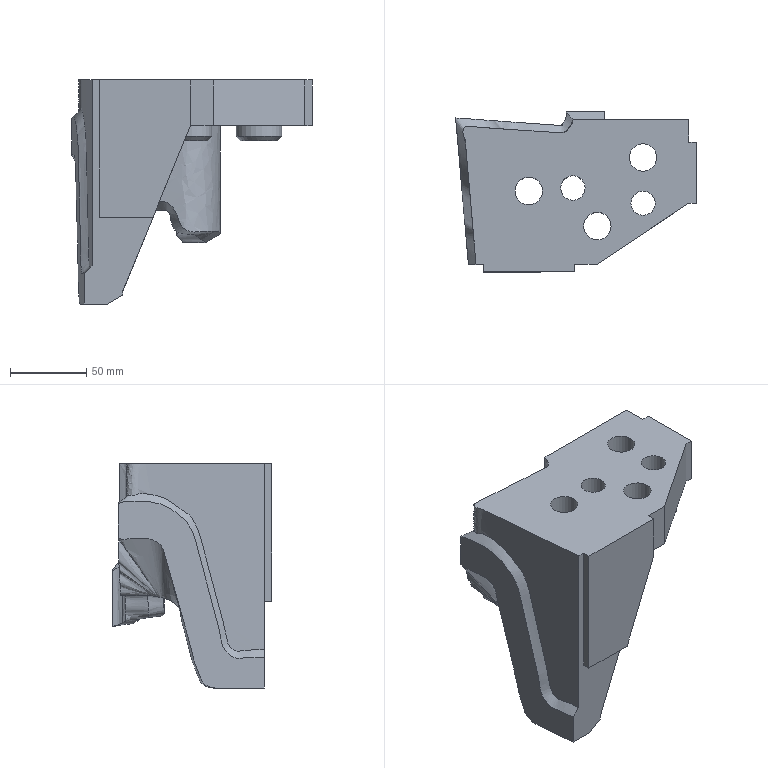Part | NX | features solid 2 | 1 solid | 45 faces | box 158 x 104.999 x 147.134 mm | volume 700826 mm3 | plane 25 | cylinder 10 | spline 8 | cone 2 | commonest cylinder face diameters 18 x3 26 x3 16 x2 30 x2